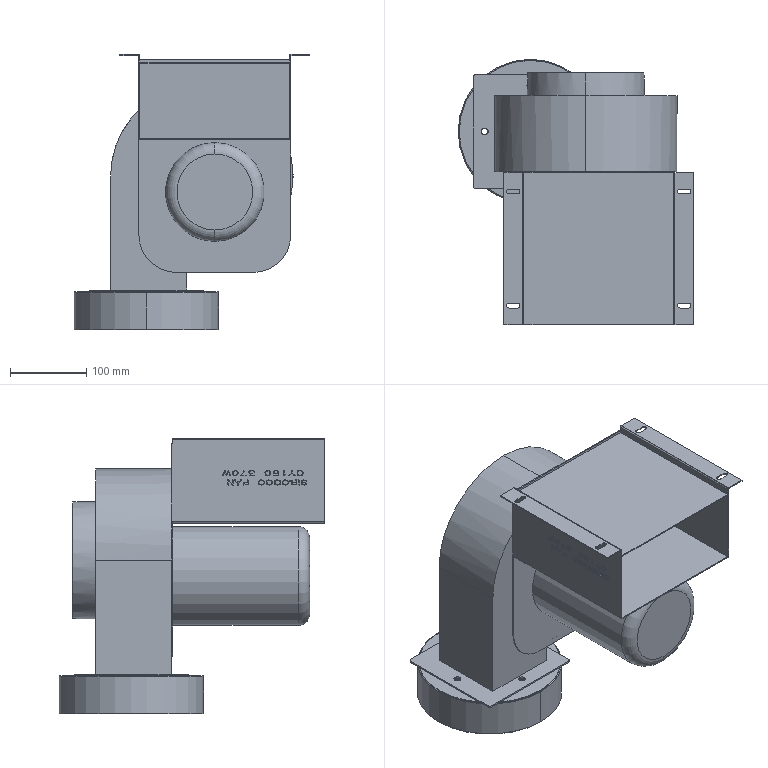Part | SolidWorks | features CompositeCurve 1 | 2 solids | 758 faces | box 310.055 x 349.5 x 362 mm | volume 816455 mm3 | plane 402 | cylinder 181 | spline 167 | torus 8 | commonest cylinder face diameters 4 x116 6.5 x12 8 x8 9 x8 0.4 x4 3.4 x4